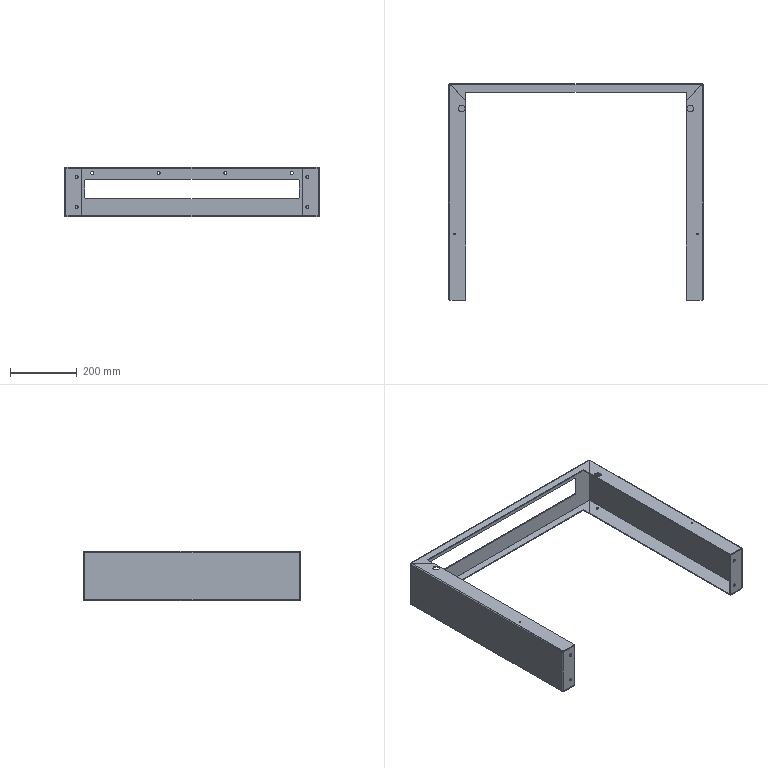Part | STEP file | HESS-408-70-15W-W-27-outer case lower support 2 | 1 solid | 126 faces | box 763 x 650 x 150 mm | volume 1289227 mm3 | plane 66 | cylinder 52 | spline 8 | commonest cylinder face diameters 9 x16 0.2 x10 6.2 x10 4.2 x4 6.8 x4 10 x4